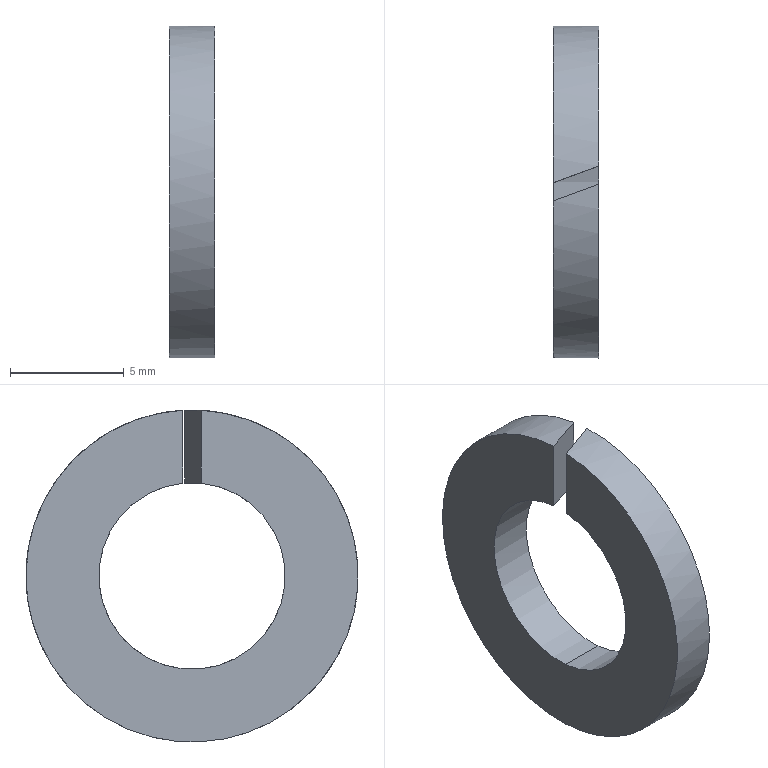Part | STEP file | KS B 1324 - No. 2 - 8 | 1 solid | 8 faces | box 2 x 14.6 x 14.6 mm | volume 224.071 mm3 | cylinder 4 | plane 4 | commonest cylinder face diameters 8.2 x2 14.6 x2
STEP:
#1=CARTESIAN_POINT('',(0.,0.,0.));
#2=DIRECTION('',(0.,0.,1.));
#3=DIRECTION('',(1.,0.,0.));
#4=AXIS2_PLACEMENT_3D('',#1,#2,#3);
#5=CARTESIAN_POINT('',(2.,1.128,3.942));
#6=VERTEX_POINT('',#5);
#7=CARTESIAN_POINT('',(0.,0.4,4.08));
#8=VERTEX_POINT('',#7);
#9=CARTESIAN_POINT('',(2.,1.128,3.942));
#10=CARTESIAN_POINT('',(1.346,0.8898,4.01));
#11=CARTESIAN_POINT('',(0.6773,0.6465,4.056));
#12=CARTESIAN_POINT('',(0.,0.4,4.08));
#13=(BOUNDED_CURVE()B_SPLINE_CURVE(3,(#9,#10,#11,#12),.UNSPECIFIED.,.F.,.F.)B_SPLINE_CURVE_WITH_KNOTS((4,4),(4.434,4.615),.PIECEWISE_BEZIER_KNOTS.)CURVE()GEOMETRIC_REPRESENTATION_ITEM()RATIONAL_B_SPLINE_CURVE((1.,0.9973,0.9973,1.))REPRESENTATION_ITEM(''));
#14=CARTESIAN_POINT('',(0.,0.,0.));
#15=DIRECTION('',(1.,0.,0.));
#16=DIRECTION('',(0.,-0.08878,-0.9961));
#17=AXIS2_PLACEMENT_3D('',#14,#15,#16);
#18=CYLINDRICAL_SURFACE('',#17,4.1);
#19=CARTESIAN_POINT('',(2.952,2.));
#20=CARTESIAN_POINT('',(2.955,1.97));
#21=CARTESIAN_POINT('',(2.96,1.911));
#22=CARTESIAN_POINT('',(2.968,1.822));
#23=CARTESIAN_POINT('',(2.976,1.732));
#24=CARTESIAN_POINT('',(2.985,1.642));
#25=CARTESIAN_POINT('',(2.993,1.552));
#26=CARTESIAN_POINT('',(3.001,1.462));
#27=CARTESIAN_POINT('',(3.009,1.372));
#28=CARTESIAN_POINT('',(3.018,1.281));
#29=CARTESIAN_POINT('',(3.026,1.191));
#30=CARTESIAN_POINT('',(3.034,1.1));
#31=CARTESIAN_POINT('',(3.042,1.009));
#32=CARTESIAN_POINT('',(3.051,0.9175));
#33=CARTESIAN_POINT('',(3.059,0.8262));
#34=CARTESIAN_POINT('',(3.067,0.7348));
#35=CARTESIAN_POINT('',(3.075,0.6432));
#36=CARTESIAN_POINT('',(3.083,0.5516));
#37=CARTESIAN_POINT('',(3.092,0.4598));
#38=CARTESIAN_POINT('',(3.1,0.368));
#39=CARTESIAN_POINT('',(3.108,0.2761));
#40=CARTESIAN_POINT('',(3.116,0.1841));
#41=CARTESIAN_POINT('',(3.125,0.09209));
#42=CARTESIAN_POINT('',(3.13,0.0307));
#43=CARTESIAN_POINT('',(3.133,0.));
#44=B_SPLINE_CURVE_WITH_KNOTS('',3,(#19,#20,#21,#22,#23,#24,#25,#26,#27,#28,#29,#30,#31,#32,#33,#34,#35,#36,#37,#38,#39,#40,#41,#42,#43),.UNSPECIFIED.,.F.,.F.,(4,1,1,1,1,1,1,1,1,1,1,1,1,1,1,1,1,1,1,1,1,1,4),(4.434,4.442,4.45,4.458,4.467,4.475,4.483,4.491,4.5,4.508,4.516,4.524,4.532,4.541,4.549,4.557,4.565,4.574,4.582,4.59,4.598,4.606,4.615),.QUASI_UNIFORM_KNOTS.);
#45=(GEOMETRIC_REPRESENTATION_CONTEXT(2)PARAMETRIC_REPRESENTATION_CONTEXT()REPRESENTATION_CONTEXT('',''));
#46=DEFINITIONAL_REPRESENTATION('',(#44),#45);
#47=PCURVE('',#18,#46);
#48=CARTESIAN_POINT('',(0.,0.4,0.));
#49=DIRECTION('',(-0.342,0.9397,0.));
#50=DIRECTION('',(0.,0.,1.));
#51=AXIS2_PLACEMENT_3D('',#48,#49,#50);
#52=PLANE('',#51);
#53=CARTESIAN_POINT('',(3.942,2.128));
#54=CARTESIAN_POINT('',(4.01,1.432));
#55=CARTESIAN_POINT('',(4.056,0.7207));
#56=CARTESIAN_POINT('',(4.08,0.));
#57=(BOUNDED_CURVE()B_SPLINE_CURVE(3,(#53,#54,#55,#56),.UNSPECIFIED.,.F.,.F.)B_SPLINE_CURVE_WITH_KNOTS((4,4),(4.434,4.615),.PIECEWISE_BEZIER_KNOTS.)CURVE()GEOMETRIC_REPRESENTATION_ITEM()RATIONAL_B_SPLINE_CURVE((1.,0.9973,0.9973,1.))REPRESENTATION_ITEM(''));
#58=(GEOMETRIC_REPRESENTATION_CONTEXT(2)PARAMETRIC_REPRESENTATION_CONTEXT()REPRESENTATION_CONTEXT('',''));
#59=DEFINITIONAL_REPRESENTATION('',(#57),#58);
#60=PCURVE('',#52,#59);
#61=SURFACE_CURVE('',#13,(#47,#60),.PCURVE_S1.);
#62=EDGE_CURVE('',#6,#8,#61,.T.);
#63=ORIENTED_EDGE('',*,*,#62,.F.);
#64=CARTESIAN_POINT('',(2.,-0.364,-4.084));
#65=VERTEX_POINT('',#64);
#66=CARTESIAN_POINT('',(2.,0.,0.));
#67=DIRECTION('',(-1.,0.,0.));
#68=DIRECTION('',(0.,-1.,0.));
#69=AXIS2_PLACEMENT_3D('',#66,#67,#68);
#70=CIRCLE('',#69,4.1);
#71=CARTESIAN_POINT('',(4.801,2.));
#72=DIRECTION('',(-1.,0.));
#73=VECTOR('',#72,1.);
#74=LINE('',#71,#73);
#75=(GEOMETRIC_REPRESENTATION_CONTEXT(2)PARAMETRIC_REPRESENTATION_CONTEXT()REPRESENTATION_CONTEXT('',''));
#76=DEFINITIONAL_REPRESENTATION('',(#74),#75);
#77=PCURVE('',#18,#76);
#78=CARTESIAN_POINT('',(2.,0.,0.));
#79=DIRECTION('',(-1.,0.,0.));
#80=DIRECTION('',(0.,0.,1.));
#81=AXIS2_PLACEMENT_3D('',#78,#79,#80);
#82=PLANE('',#81);
#83=CARTESIAN_POINT('',(0.,0.));
#84=DIRECTION('',(0.,-1.));
#85=AXIS2_PLACEMENT_2D('',#83,#84);
#86=CIRCLE('',#85,4.1);
#87=(GEOMETRIC_REPRESENTATION_CONTEXT(2)PARAMETRIC_REPRESENTATION_CONTEXT()REPRESENTATION_CONTEXT('',''));
#88=DEFINITIONAL_REPRESENTATION('',(#86),#87);
#89=PCURVE('',#82,#88);
#90=SURFACE_CURVE('',#70,(#77,#89),.PCURVE_S1.);
#91=EDGE_CURVE('',#6,#65,#90,.T.);
#92=ORIENTED_EDGE('',*,*,#91,.T.);
#93=CARTESIAN_POINT('',(0.,-0.364,-4.084));
#94=VERTEX_POINT('',#93);
#95=CARTESIAN_POINT('',(0.,-0.364,-4.084));
#96=DIRECTION('',(1.,0.,0.));
#97=VECTOR('',#96,1.);
#98=LINE('',#95,#97);
#99=CARTESIAN_POINT('',(0.,0.));
#100=DIRECTION('',(0.,1.));
#101=VECTOR('',#100,1.);
#102=LINE('',#99,#101);
#103=(GEOMETRIC_REPRESENTATION_CONTEXT(2)PARAMETRIC_REPRESENTATION_CONTEXT()REPRESENTATION_CONTEXT('',''));
#104=DEFINITIONAL_REPRESENTATION('',(#102),#103);
#105=PCURVE('',#18,#104);
#106=CARTESIAN_POINT('',(0.,0.,0.));
#107=DIRECTION('',(1.,0.,0.));
#108=DIRECTION('',(0.,-0.08878,-0.9961));
#109=AXIS2_PLACEMENT_3D('',#106,#107,#108);
#110=CYLINDRICAL_SURFACE('',#109,4.1);
#111=CARTESIAN_POINT('',(6.283,0.));
#112=DIRECTION('',(0.,1.));
#113=VECTOR('',#112,1.);
#114=LINE('',#111,#113);
#115=(GEOMETRIC_REPRESENTATION_CONTEXT(2)PARAMETRIC_REPRESENTATION_CONTEXT()REPRESENTATION_CONTEXT('',''));
#116=DEFINITIONAL_REPRESENTATION('',(#114),#115);
#117=PCURVE('',#110,#116);
#118=SURFACE_CURVE('',#98,(#105,#117),.PCURVE_S1.);
#119=EDGE_CURVE('',#94,#65,#118,.T.);
#120=ORIENTED_EDGE('',*,*,#119,.F.);
#121=CARTESIAN_POINT('',(0.,0.,0.));
#122=DIRECTION('',(1.,0.,0.));
#123=DIRECTION('',(0.,-1.,0.));
#124=AXIS2_PLACEMENT_3D('',#121,#122,#123);
#125=CIRCLE('',#124,4.1);
#126=CARTESIAN_POINT('',(-1.482,0.));
#127=DIRECTION('',(1.,0.));
#128=VECTOR('',#127,1.);
#129=LINE('',#126,#128);
#130=(GEOMETRIC_REPRESENTATION_CONTEXT(2)PARAMETRIC_REPRESENTATION_CONTEXT()REPRESENTATION_CONTEXT('',''));
#131=DEFINITIONAL_REPRESENTATION('',(#129),#130);
#132=PCURVE('',#18,#131);
#133=CARTESIAN_POINT('',(0.,0.,0.));
#134=DIRECTION('',(-1.,0.,0.));
#135=DIRECTION('',(0.,0.,1.));
#136=AXIS2_PLACEMENT_3D('',#133,#134,#135);
#137=PLANE('',#136);
#138=CARTESIAN_POINT('',(0.,-4.1));
#139=CARTESIAN_POINT('',(-7.101,-4.1));
#140=CARTESIAN_POINT('',(-3.551,2.05));
#141=CARTESIAN_POINT('',(0.,8.2));
#142=CARTESIAN_POINT('',(3.551,2.05));
#143=CARTESIAN_POINT('',(7.101,-4.1));
#144=CARTESIAN_POINT('',(0.,-4.1));
#145=(BOUNDED_CURVE()B_SPLINE_CURVE(2,(#138,#139,#140,#141,#142,#143,#144),.UNSPECIFIED.,.T.,.F.)B_SPLINE_CURVE_WITH_KNOTS((1,2,2,2,2,1),(-2.094,0.,2.094,4.189,6.283,8.378),.UNSPECIFIED.)CURVE()GEOMETRIC_REPRESENTATION_ITEM()RATIONAL_B_SPLINE_CURVE((1.,0.5,1.,0.5,1.,0.5,1.))REPRESENTATION_ITEM(''));
#146=(GEOMETRIC_REPRESENTATION_CONTEXT(2)PARAMETRIC_REPRESENTATION_CONTEXT()REPRESENTATION_CONTEXT('',''));
#147=DEFINITIONAL_REPRESENTATION('',(#145),#146);
#148=PCURVE('',#137,#147);
#149=SURFACE_CURVE('',#125,(#132,#148),.PCURVE_S1.);
#150=EDGE_CURVE('',#94,#8,#149,.T.);
#151=ORIENTED_EDGE('',*,*,#150,.T.);
#152=EDGE_LOOP('',(#63,#92,#120,#151));
#153=FACE_BOUND('',#152,.F.);
#154=ADVANCED_FACE('',(#153),#18,.F.);
#155=CARTESIAN_POINT('',(0.,-0.364,-7.291));
#156=VERTEX_POINT('',#155);
#157=CARTESIAN_POINT('',(0.,-0.4,7.289));
#158=VERTEX_POINT('',#157);
#159=CARTESIAN_POINT('',(0.,0.,0.));
#160=DIRECTION('',(-1.,0.,0.));
#161=DIRECTION('',(0.,-1.,0.));
#162=AXIS2_PLACEMENT_3D('',#159,#160,#161);
#163=CIRCLE('',#162,7.3);
#164=CARTESIAN_POINT('',(0.,0.,0.));
#165=DIRECTION('',(1.,0.,0.));
#166=DIRECTION('',(0.,-0.04986,-0.9988));
#167=AXIS2_PLACEMENT_3D('',#164,#165,#166);
#168=CYLINDRICAL_SURFACE('',#167,7.3);
#169=CARTESIAN_POINT('',(11.045,0.));
#170=DIRECTION('',(-1.,0.));
#171=VECTOR('',#170,1.);
#172=LINE('',#169,#171);
#173=(GEOMETRIC_REPRESENTATION_CONTEXT(2)PARAMETRIC_REPRESENTATION_CONTEXT()REPRESENTATION_CONTEXT('',''));
#174=DEFINITIONAL_REPRESENTATION('',(#172),#173);
#175=PCURVE('',#168,#174);
#176=CARTESIAN_POINT('',(0.,0.));
#177=DIRECTION('',(0.,-1.));
#178=AXIS2_PLACEMENT_2D('',#176,#177);
#179=CIRCLE('',#178,7.3);
#180=(GEOMETRIC_REPRESENTATION_CONTEXT(2)PARAMETRIC_REPRESENTATION_CONTEXT()REPRESENTATION_CONTEXT('',''));
#181=DEFINITIONAL_REPRESENTATION('',(#179),#180);
#182=PCURVE('',#137,#181);
#183=SURFACE_CURVE('',#163,(#175,#182),.PCURVE_S1.);
#184=EDGE_CURVE('',#156,#158,#183,.T.);
#185=ORIENTED_EDGE('',*,*,#184,.F.);
#186=CARTESIAN_POINT('',(2.,-0.364,-7.291));
#187=VERTEX_POINT('',#186);
#188=CARTESIAN_POINT('',(0.,-0.364,-7.291));
#189=DIRECTION('',(1.,0.,0.));
#190=VECTOR('',#189,1.);
#191=LINE('',#188,#190);
#192=CARTESIAN_POINT('',(6.283,0.));
#193=DIRECTION('',(0.,1.));
#194=VECTOR('',#193,1.);
#195=LINE('',#192,#194);
#196=(GEOMETRIC_REPRESENTATION_CONTEXT(2)PARAMETRIC_REPRESENTATION_CONTEXT()REPRESENTATION_CONTEXT('',''));
#197=DEFINITIONAL_REPRESENTATION('',(#195),#196);
#198=PCURVE('',#168,#197);
#199=CARTESIAN_POINT('',(0.,0.,0.));
#200=DIRECTION('',(1.,0.,0.));
#201=DIRECTION('',(0.,-0.04986,-0.9988));
#202=AXIS2_PLACEMENT_3D('',#199,#200,#201);
#203=CYLINDRICAL_SURFACE('',#202,7.3);
#204=CARTESIAN_POINT('',(0.,0.));
#205=DIRECTION('',(0.,1.));
#206=VECTOR('',#205,1.);
#207=LINE('',#204,#206);
#208=(GEOMETRIC_REPRESENTATION_CONTEXT(2)PARAMETRIC_REPRESENTATION_CONTEXT()REPRESENTATION_CONTEXT('',''));
#209=DEFINITIONAL_REPRESENTATION('',(#207),#208);
#210=PCURVE('',#203,#209);
#211=SURFACE_CURVE('',#191,(#198,#210),.PCURVE_S1.);
#212=EDGE_CURVE('',#156,#187,#211,.T.);
#213=ORIENTED_EDGE('',*,*,#212,.T.);
#214=CARTESIAN_POINT('',(2.,0.3279,7.293));
#215=VERTEX_POINT('',#214);
#216=CARTESIAN_POINT('',(2.,0.,0.));
#217=DIRECTION('',(-1.,0.,0.));
#218=DIRECTION('',(0.,-1.,0.));
#219=AXIS2_PLACEMENT_3D('',#216,#217,#218);
#220=CIRCLE('',#219,7.3);
#221=CARTESIAN_POINT('',(11.045,2.));
#222=DIRECTION('',(-1.,0.));
#223=VECTOR('',#222,1.);
#224=LINE('',#221,#223);
#225=(GEOMETRIC_REPRESENTATION_CONTEXT(2)PARAMETRIC_REPRESENTATION_CONTEXT()REPRESENTATION_CONTEXT('',''));
#226=DEFINITIONAL_REPRESENTATION('',(#224),#225);
#227=PCURVE('',#168,#226);
#228=CARTESIAN_POINT('',(0.,0.));
#229=DIRECTION('',(0.,-1.));
#230=AXIS2_PLACEMENT_2D('',#228,#229);
#231=CIRCLE('',#230,7.3);
#232=(GEOMETRIC_REPRESENTATION_CONTEXT(2)PARAMETRIC_REPRESENTATION_CONTEXT()REPRESENTATION_CONTEXT('',''));
#233=DEFINITIONAL_REPRESENTATION('',(#231),#232);
#234=PCURVE('',#82,#233);
#235=SURFACE_CURVE('',#220,(#227,#234),.PCURVE_S1.);
#236=EDGE_CURVE('',#187,#215,#235,.T.);
#237=ORIENTED_EDGE('',*,*,#236,.T.);
#238=CARTESIAN_POINT('',(2.,0.3279,7.293));
#239=CARTESIAN_POINT('',(1.333,0.08533,7.304));
#240=CARTESIAN_POINT('',(0.6662,-0.1575,7.302));
#241=CARTESIAN_POINT('',(0.,-0.4,7.289));
#242=(BOUNDED_CURVE()B_SPLINE_CURVE(3,(#238,#239,#240,#241),.UNSPECIFIED.,.F.,.F.)B_SPLINE_CURVE_WITH_KNOTS((4,4),(4.667,4.767),.PIECEWISE_BEZIER_KNOTS.)CURVE()GEOMETRIC_REPRESENTATION_ITEM()RATIONAL_B_SPLINE_CURVE((1.,0.9992,0.9992,1.))REPRESENTATION_ITEM(''));
#243=CARTESIAN_POINT('',(3.147,2.));
#244=CARTESIAN_POINT('',(3.148,1.97));
#245=CARTESIAN_POINT('',(3.151,1.909));
#246=CARTESIAN_POINT('',(3.156,1.818));
#247=CARTESIAN_POINT('',(3.16,1.727));
#248=CARTESIAN_POINT('',(3.165,1.637));
#249=CARTESIAN_POINT('',(3.169,1.546));
#250=CARTESIAN_POINT('',(3.174,1.455));
#251=CARTESIAN_POINT('',(3.178,1.364));
#252=CARTESIAN_POINT('',(3.183,1.273));
#253=CARTESIAN_POINT('',(3.187,1.182));
#254=CARTESIAN_POINT('',(3.192,1.091));
#255=CARTESIAN_POINT('',(3.196,0.9999));
#256=CARTESIAN_POINT('',(3.201,0.9089));
#257=CARTESIAN_POINT('',(3.205,0.818));
#258=CARTESIAN_POINT('',(3.21,0.727));
#259=CARTESIAN_POINT('',(3.215,0.6361));
#260=CARTESIAN_POINT('',(3.219,0.5451));
#261=CARTESIAN_POINT('',(3.224,0.4542));
#262=CARTESIAN_POINT('',(3.228,0.3633));
#263=CARTESIAN_POINT('',(3.233,0.2725));
#264=CARTESIAN_POINT('',(3.237,0.1816));
#265=CARTESIAN_POINT('',(3.242,0.09078));
#266=CARTESIAN_POINT('',(3.245,0.03026));
#267=CARTESIAN_POINT('',(3.246,0.));
#268=B_SPLINE_CURVE_WITH_KNOTS('',3,(#243,#244,#245,#246,#247,#248,#249,#250,#251,#252,#253,#254,#255,#256,#257,#258,#259,#260,#261,#262,#263,#264,#265,#266,#267),.UNSPECIFIED.,.F.,.F.,(4,1,1,1,1,1,1,1,1,1,1,1,1,1,1,1,1,1,1,1,1,1,4),(4.667,4.672,4.677,4.681,4.686,4.69,4.695,4.699,4.704,4.708,4.713,4.717,4.722,4.726,4.731,4.735,4.74,4.745,4.749,4.754,4.758,4.763,4.767),.QUASI_UNIFORM_KNOTS.);
#269=(GEOMETRIC_REPRESENTATION_CONTEXT(2)PARAMETRIC_REPRESENTATION_CONTEXT()REPRESENTATION_CONTEXT('',''));
#270=DEFINITIONAL_REPRESENTATION('',(#268),#269);
#271=PCURVE('',#168,#270);
#272=CARTESIAN_POINT('',(2.,0.3279,0.));
#273=DIRECTION('',(0.342,-0.9397,0.));
#274=DIRECTION('',(0.,0.,-1.));
#275=AXIS2_PLACEMENT_3D('',#272,#273,#274);
#276=PLANE('',#275);
#277=CARTESIAN_POINT('',(-7.293,0.));
#278=CARTESIAN_POINT('',(-7.304,-0.7093));
#279=CARTESIAN_POINT('',(-7.302,-1.419));
#280=CARTESIAN_POINT('',(-7.289,-2.128));
#281=(BOUNDED_CURVE()B_SPLINE_CURVE(3,(#277,#278,#279,#280),.UNSPECIFIED.,.F.,.F.)B_SPLINE_CURVE_WITH_KNOTS((4,4),(4.667,4.767),.PIECEWISE_BEZIER_KNOTS.)CURVE()GEOMETRIC_REPRESENTATION_ITEM()RATIONAL_B_SPLINE_CURVE((1.,0.9992,0.9992,1.))REPRESENTATION_ITEM(''));
#282=(GEOMETRIC_REPRESENTATION_CONTEXT(2)PARAMETRIC_REPRESENTATION_CONTEXT()REPRESENTATION_CONTEXT('',''));
#283=DEFINITIONAL_REPRESENTATION('',(#281),#282);
#284=PCURVE('',#276,#283);
#285=SURFACE_CURVE('',#242,(#271,#284),.PCURVE_S1.);
#286=EDGE_CURVE('',#215,#158,#285,.T.);
#287=ORIENTED_EDGE('',*,*,#286,.T.);
#288=EDGE_LOOP('',(#185,#213,#237,#287));
#289=FACE_BOUND('',#288,.T.);
#290=ADVANCED_FACE('',(#289),#168,.T.);
#291=CARTESIAN_POINT('',(0.,-0.4,4.08));
#292=VERTEX_POINT('',#291);
#293=CARTESIAN_POINT('',(0.,-0.4,0.));
#294=DIRECTION('',(0.,0.,-1.));
#295=VECTOR('',#294,1.);
#296=LINE('',#293,#295);
#297=CARTESIAN_POINT('',(0.,-0.4));
#298=DIRECTION('',(-1.,0.));
#299=VECTOR('',#298,1.);
#300=LINE('',#297,#299);
#301=(GEOMETRIC_REPRESENTATION_CONTEXT(2)PARAMETRIC_REPRESENTATION_CONTEXT()REPRESENTATION_CONTEXT('',''));
#302=DEFINITIONAL_REPRESENTATION('',(#300),#301);
#303=PCURVE('',#137,#302);
#304=CARTESIAN_POINT('',(0.,-2.128));
#305=DIRECTION('',(1.,0.));
#306=VECTOR('',#305,1.);
#307=LINE('',#304,#306);
#308=(GEOMETRIC_REPRESENTATION_CONTEXT(2)PARAMETRIC_REPRESENTATION_CONTEXT()REPRESENTATION_CONTEXT('',''));
#309=DEFINITIONAL_REPRESENTATION('',(#307),#308);
#310=PCURVE('',#276,#309);
#311=SURFACE_CURVE('',#296,(#303,#310),.PCURVE_S1.);
#312=EDGE_CURVE('',#158,#292,#311,.T.);
#313=ORIENTED_EDGE('',*,*,#312,.T.);
#314=CARTESIAN_POINT('',(0.,0.,0.));
#315=DIRECTION('',(1.,0.,0.));
#316=DIRECTION('',(0.,-1.,0.));
#317=AXIS2_PLACEMENT_3D('',#314,#315,#316);
#318=CIRCLE('',#317,4.1);
#319=CARTESIAN_POINT('',(0.,-4.1));
#320=CARTESIAN_POINT('',(-7.101,-4.1));
#321=CARTESIAN_POINT('',(-3.551,2.05));
#322=CARTESIAN_POINT('',(0.,8.2));
#323=CARTESIAN_POINT('',(3.551,2.05));
#324=CARTESIAN_POINT('',(7.101,-4.1));
#325=CARTESIAN_POINT('',(0.,-4.1));
#326=(BOUNDED_CURVE()B_SPLINE_CURVE(2,(#319,#320,#321,#322,#323,#324,#325),.UNSPECIFIED.,.T.,.F.)B_SPLINE_CURVE_WITH_KNOTS((1,2,2,2,2,1),(-2.094,0.,2.094,4.189,6.283,8.378),.UNSPECIFIED.)CURVE()GEOMETRIC_REPRESENTATION_ITEM()RATIONAL_B_SPLINE_CURVE((1.,0.5,1.,0.5,1.,0.5,1.))REPRESENTATION_ITEM(''));
#327=(GEOMETRIC_REPRESENTATION_CONTEXT(2)PARAMETRIC_REPRESENTATION_CONTEXT()REPRESENTATION_CONTEXT('',''));
#328=DEFINITIONAL_REPRESENTATION('',(#326),#327);
#329=PCURVE('',#137,#328);
#330=CARTESIAN_POINT('',(-1.482,0.));
#331=DIRECTION('',(1.,0.));
#332=VECTOR('',#331,1.);
#333=LINE('',#330,#332);
#334=(GEOMETRIC_REPRESENTATION_CONTEXT(2)PARAMETRIC_REPRESENTATION_CONTEXT()REPRESENTATION_CONTEXT('',''));
#335=DEFINITIONAL_REPRESENTATION('',(#333),#334);
#336=PCURVE('',#110,#335);
#337=SURFACE_CURVE('',#318,(#329,#336),.PCURVE_S1.);
#338=EDGE_CURVE('',#292,#94,#337,.T.);
#339=ORIENTED_EDGE('',*,*,#338,.T.);
#340=ORIENTED_EDGE('',*,*,#150,.T.);
#341=CARTESIAN_POINT('',(0.,0.4,7.289));
#342=VERTEX_POINT('',#341);
#343=CARTESIAN_POINT('',(0.,0.4,0.));
#344=DIRECTION('',(0.,0.,1.));
#345=VECTOR('',#344,1.);
#346=LINE('',#343,#345);
#347=CARTESIAN_POINT('',(0.,0.4));
#348=DIRECTION('',(1.,0.));
#349=VECTOR('',#348,1.);
#350=LINE('',#347,#349);
#351=(GEOMETRIC_REPRESENTATION_CONTEXT(2)PARAMETRIC_REPRESENTATION_CONTEXT()REPRESENTATION_CONTEXT('',''));
#352=DEFINITIONAL_REPRESENTATION('',(#350),#351);
#353=PCURVE('',#137,#352);
#354=CARTESIAN_POINT('',(0.,0.));
#355=DIRECTION('',(1.,0.));
#356=VECTOR('',#355,1.);
#357=LINE('',#354,#356);
#358=(GEOMETRIC_REPRESENTATION_CONTEXT(2)PARAMETRIC_REPRESENTATION_CONTEXT()REPRESENTATION_CONTEXT('',''));
#359=DEFINITIONAL_REPRESENTATION('',(#357),#358);
#360=PCURVE('',#52,#359);
#361=SURFACE_CURVE('',#346,(#353,#360),.PCURVE_S1.);
#362=EDGE_CURVE('',#8,#342,#361,.T.);
#363=ORIENTED_EDGE('',*,*,#362,.T.);
#364=CARTESIAN_POINT('',(0.,0.,0.));
#365=DIRECTION('',(-1.,0.,0.));
#366=DIRECTION('',(0.,-1.,0.));
#367=AXIS2_PLACEMENT_3D('',#364,#365,#366);
#368=CIRCLE('',#367,7.3);
#369=CARTESIAN_POINT('',(0.,0.));
#370=DIRECTION('',(0.,-1.));
#371=AXIS2_PLACEMENT_2D('',#369,#370);
#372=CIRCLE('',#371,7.3);
#373=(GEOMETRIC_REPRESENTATION_CONTEXT(2)PARAMETRIC_REPRESENTATION_CONTEXT()REPRESENTATION_CONTEXT('',''));
#374=DEFINITIONAL_REPRESENTATION('',(#372),#373);
#375=PCURVE('',#137,#374);
#376=CARTESIAN_POINT('',(4.762,0.));
#377=DIRECTION('',(-1.,0.));
#378=VECTOR('',#377,1.);
#379=LINE('',#376,#378);
#380=(GEOMETRIC_REPRESENTATION_CONTEXT(2)PARAMETRIC_REPRESENTATION_CONTEXT()REPRESENTATION_CONTEXT('',''));
#381=DEFINITIONAL_REPRESENTATION('',(#379),#380);
#382=PCURVE('',#203,#381);
#383=SURFACE_CURVE('',#368,(#375,#382),.PCURVE_S1.);
#384=EDGE_CURVE('',#342,#156,#383,.T.);
#385=ORIENTED_EDGE('',*,*,#384,.T.);
#386=ORIENTED_EDGE('',*,*,#184,.T.);
#387=EDGE_LOOP('',(#313,#339,#340,#363,#385,#386));
#388=FACE_BOUND('',#387,.T.);
#389=ADVANCED_FACE('',(#388),#137,.T.);
#390=ORIENTED_EDGE('',*,*,#212,.F.);
#391=ORIENTED_EDGE('',*,*,#384,.F.);
#392=CARTESIAN_POINT('',(2.,1.128,7.212));
#393=VERTEX_POINT('',#392);
#394=CARTESIAN_POINT('',(0.,0.4,7.289));
#395=CARTESIAN_POINT('',(0.6699,0.6438,7.276));
#396=CARTESIAN_POINT('',(1.337,0.8867,7.25));
#397=CARTESIAN_POINT('',(2.,1.128,7.212));
#398=(BOUNDED_CURVE()B_SPLINE_CURVE(3,(#394,#395,#396,#397),.UNSPECIFIED.,.F.,.F.)B_SPLINE_CURVE_WITH_KNOTS((4,4),(1.626,1.726),.PIECEWISE_BEZIER_KNOTS.)CURVE()GEOMETRIC_REPRESENTATION_ITEM()RATIONAL_B_SPLINE_CURVE((1.,0.9992,0.9992,1.))REPRESENTATION_ITEM(''));
#399=CARTESIAN_POINT('',(3.137,0.));
#400=CARTESIAN_POINT('',(3.135,0.03042));
#401=CARTESIAN_POINT('',(3.132,0.09127));
#402=CARTESIAN_POINT('',(3.128,0.1825));
#403=CARTESIAN_POINT('',(3.123,0.2738));
#404=CARTESIAN_POINT('',(3.118,0.365));
#405=CARTESIAN_POINT('',(3.114,0.4562));
#406=CARTESIAN_POINT('',(3.109,0.5473));
#407=CARTESIAN_POINT('',(3.105,0.6385));
#408=CARTESIAN_POINT('',(3.1,0.7296));
#409=CARTESIAN_POINT('',(3.096,0.8206));
#410=CARTESIAN_POINT('',(3.091,0.9117));
#411=CARTESIAN_POINT('',(3.086,1.003));
#412=CARTESIAN_POINT('',(3.082,1.094));
#413=CARTESIAN_POINT('',(3.077,1.184));
#414=CARTESIAN_POINT('',(3.073,1.275));
#415=CARTESIAN_POINT('',(3.068,1.366));
#416=CARTESIAN_POINT('',(3.064,1.457));
#417=CARTESIAN_POINT('',(3.059,1.548));
#418=CARTESIAN_POINT('',(3.055,1.638));
#419=CARTESIAN_POINT('',(3.05,1.729));
#420=CARTESIAN_POINT('',(3.045,1.819));
#421=CARTESIAN_POINT('',(3.041,1.91));
#422=CARTESIAN_POINT('',(3.038,1.97));
#423=CARTESIAN_POINT('',(3.036,2.));
#424=B_SPLINE_CURVE_WITH_KNOTS('',3,(#399,#400,#401,#402,#403,#404,#405,#406,#407,#408,#409,#410,#411,#412,#413,#414,#415,#416,#417,#418,#419,#420,#421,#422,#423),.UNSPECIFIED.,.F.,.F.,(4,1,1,1,1,1,1,1,1,1,1,1,1,1,1,1,1,1,1,1,1,1,4),(1.626,1.63,1.635,1.639,1.644,1.648,1.653,1.658,1.662,1.667,1.671,1.676,1.68,1.685,1.689,1.694,1.699,1.703,1.708,1.712,1.717,1.721,1.726),.QUASI_UNIFORM_KNOTS.);
#425=(GEOMETRIC_REPRESENTATION_CONTEXT(2)PARAMETRIC_REPRESENTATION_CONTEXT()REPRESENTATION_CONTEXT('',''));
#426=DEFINITIONAL_REPRESENTATION('',(#424),#425);
#427=PCURVE('',#203,#426);
#428=CARTESIAN_POINT('',(7.289,0.));
#429=CARTESIAN_POINT('',(7.276,0.7129));
#430=CARTESIAN_POINT('',(7.25,1.423));
#431=CARTESIAN_POINT('',(7.212,2.128));
#432=(BOUNDED_CURVE()B_SPLINE_CURVE(3,(#428,#429,#430,#431),.UNSPECIFIED.,.F.,.F.)B_SPLINE_CURVE_WITH_KNOTS((4,4),(1.626,1.726),.PIECEWISE_BEZIER_KNOTS.)CURVE()GEOMETRIC_REPRESENTATION_ITEM()RATIONAL_B_SPLINE_CURVE((1.,0.9992,0.9992,1.))REPRESENTATION_ITEM(''));
#433=(GEOMETRIC_REPRESENTATION_CONTEXT(2)PARAMETRIC_REPRESENTATION_CONTEXT()REPRESENTATION_CONTEXT('',''));
#434=DEFINITIONAL_REPRESENTATION('',(#432),#433);
#435=PCURVE('',#52,#434);
#436=SURFACE_CURVE('',#398,(#427,#435),.PCURVE_S1.);
#437=EDGE_CURVE('',#342,#393,#436,.T.);
#438=ORIENTED_EDGE('',*,*,#437,.T.);
#439=CARTESIAN_POINT('',(2.,0.,0.));
#440=DIRECTION('',(-1.,0.,0.));
#441=DIRECTION('',(0.,-1.,0.));
#442=AXIS2_PLACEMENT_3D('',#439,#440,#441);
#443=CIRCLE('',#442,7.3);
#444=CARTESIAN_POINT('',(4.762,2.));
#445=DIRECTION('',(-1.,0.));
#446=VECTOR('',#445,1.);
#447=LINE('',#444,#446);
#448=(GEOMETRIC_REPRESENTATION_CONTEXT(2)PARAMETRIC_REPRESENTATION_CONTEXT()REPRESENTATION_CONTEXT('',''));
#449=DEFINITIONAL_REPRESENTATION('',(#447),#448);
#450=PCURVE('',#203,#449);
#451=CARTESIAN_POINT('',(0.,0.));
#452=DIRECTION('',(0.,-1.));
#453=AXIS2_PLACEMENT_2D('',#451,#452);
#454=CIRCLE('',#453,7.3);
#455=(GEOMETRIC_REPRESENTATION_CONTEXT(2)PARAMETRIC_REPRESENTATION_CONTEXT()REPRESENTATION_CONTEXT('',''));
#456=DEFINITIONAL_REPRESENTATION('',(#454),#455);
#457=PCURVE('',#82,#456);
#458=SURFACE_CURVE('',#443,(#450,#457),.PCURVE_S1.);
#459=EDGE_CURVE('',#393,#187,#458,.T.);
#460=ORIENTED_EDGE('',*,*,#459,.T.);
#461=EDGE_LOOP('',(#390,#391,#438,#460));
#462=FACE_BOUND('',#461,.T.);
#463=ADVANCED_FACE('',(#462),#203,.T.);
#464=CARTESIAN_POINT('',(2.,0.3279,4.087));
#465=VERTEX_POINT('',#464);
#466=CARTESIAN_POINT('',(2.,0.,0.));
#467=DIRECTION('',(-1.,0.,0.));
#468=DIRECTION('',(0.,-1.,0.));
#469=AXIS2_PLACEMENT_3D('',#466,#467,#468);
#470=CIRCLE('',#469,4.1);
#471=CARTESIAN_POINT('',(11.084,2.));
#472=DIRECTION('',(-1.,0.));
#473=VECTOR('',#472,1.);
#474=LINE('',#471,#473);
#475=(GEOMETRIC_REPRESENTATION_CONTEXT(2)PARAMETRIC_REPRESENTATION_CONTEXT()REPRESENTATION_CONTEXT('',''));
#476=DEFINITIONAL_REPRESENTATION('',(#474),#475);
#477=PCURVE('',#110,#476);
#478=CARTESIAN_POINT('',(0.,0.));
#479=DIRECTION('',(0.,-1.));
#480=AXIS2_PLACEMENT_2D('',#478,#479);
#481=CIRCLE('',#480,4.1);
#482=(GEOMETRIC_REPRESENTATION_CONTEXT(2)PARAMETRIC_REPRESENTATION_CONTEXT()REPRESENTATION_CONTEXT('',''));
#483=DEFINITIONAL_REPRESENTATION('',(#481),#482);
#484=PCURVE('',#82,#483);
#485=SURFACE_CURVE('',#470,(#477,#484),.PCURVE_S1.);
#486=EDGE_CURVE('',#65,#465,#485,.T.);
#487=ORIENTED_EDGE('',*,*,#486,.T.);
#488=CARTESIAN_POINT('',(0.,-0.4,4.08));
#489=CARTESIAN_POINT('',(0.6653,-0.1579,4.104));
#490=CARTESIAN_POINT('',(1.334,0.08542,4.106));
#491=CARTESIAN_POINT('',(2.,0.3279,4.087));
#492=(BOUNDED_CURVE()B_SPLINE_CURVE(3,(#488,#489,#490,#491),.UNSPECIFIED.,.F.,.F.)B_SPLINE_CURVE_WITH_KNOTS((4,4),(1.473,1.651),.PIECEWISE_BEZIER_KNOTS.)CURVE()GEOMETRIC_REPRESENTATION_ITEM()RATIONAL_B_SPLINE_CURVE((1.,0.9974,0.9974,1.))REPRESENTATION_ITEM(''));
#493=CARTESIAN_POINT('',(3.328,0.));
#494=CARTESIAN_POINT('',(3.326,0.03016));
#495=CARTESIAN_POINT('',(3.32,0.09051));
#496=CARTESIAN_POINT('',(3.312,0.1811));
#497=CARTESIAN_POINT('',(3.304,0.2719));
#498=CARTESIAN_POINT('',(3.296,0.3626));
#499=CARTESIAN_POINT('',(3.288,0.4535));
#500=CARTESIAN_POINT('',(3.28,0.5444));
#501=CARTESIAN_POINT('',(3.272,0.6354));
#502=CARTESIAN_POINT('',(3.264,0.7264));
#503=CARTESIAN_POINT('',(3.255,0.8175));
#504=CARTESIAN_POINT('',(3.247,0.9085));
#505=CARTESIAN_POINT('',(3.239,0.9996));
#506=CARTESIAN_POINT('',(3.231,1.091));
#507=CARTESIAN_POINT('',(3.223,1.182));
#508=CARTESIAN_POINT('',(3.215,1.273));
#509=CARTESIAN_POINT('',(3.207,1.364));
#510=CARTESIAN_POINT('',(3.199,1.455));
#511=CARTESIAN_POINT('',(3.191,1.546));
#512=CARTESIAN_POINT('',(3.183,1.637));
#513=CARTESIAN_POINT('',(3.175,1.728));
#514=CARTESIAN_POINT('',(3.167,1.819));
#515=CARTESIAN_POINT('',(3.158,1.909));
#516=CARTESIAN_POINT('',(3.153,1.97));
#517=CARTESIAN_POINT('',(3.15,2.));
#518=B_SPLINE_CURVE_WITH_KNOTS('',3,(#493,#494,#495,#496,#497,#498,#499,#500,#501,#502,#503,#504,#505,#506,#507,#508,#509,#510,#511,#512,#513,#514,#515,#516,#517),.UNSPECIFIED.,.F.,.F.,(4,1,1,1,1,1,1,1,1,1,1,1,1,1,1,1,1,1,1,1,1,1,4),(1.473,1.481,1.489,1.497,1.505,1.513,1.522,1.53,1.538,1.546,1.554,1.562,1.57,1.578,1.586,1.594,1.602,1.61,1.619,1.627,1.635,1.643,1.651),.QUASI_UNIFORM_KNOTS.);
#519=(GEOMETRIC_REPRESENTATION_CONTEXT(2)PARAMETRIC_REPRESENTATION_CONTEXT()REPRESENTATION_CONTEXT('',''));
#520=DEFINITIONAL_REPRESENTATION('',(#518),#519);
#521=PCURVE('',#110,#520);
#522=CARTESIAN_POINT('',(-4.08,-2.128));
#523=CARTESIAN_POINT('',(-4.104,-1.42));
#524=CARTESIAN_POINT('',(-4.106,-0.7091));
#525=CARTESIAN_POINT('',(-4.087,0.));
#526=(BOUNDED_CURVE()B_SPLINE_CURVE(3,(#522,#523,#524,#525),.UNSPECIFIED.,.F.,.F.)B_SPLINE_CURVE_WITH_KNOTS((4,4),(1.473,1.651),.PIECEWISE_BEZIER_KNOTS.)CURVE()GEOMETRIC_REPRESENTATION_ITEM()RATIONAL_B_SPLINE_CURVE((1.,0.9974,0.9974,1.))REPRESENTATION_ITEM(''));
#527=(GEOMETRIC_REPRESENTATION_CONTEXT(2)PARAMETRIC_REPRESENTATION_CONTEXT()REPRESENTATION_CONTEXT('',''));
#528=DEFINITIONAL_REPRESENTATION('',(#526),#527);
#529=PCURVE('',#276,#528);
#530=SURFACE_CURVE('',#492,(#521,#529),.PCURVE_S1.);
#531=EDGE_CURVE('',#292,#465,#530,.T.);
#532=ORIENTED_EDGE('',*,*,#531,.F.);
#533=ORIENTED_EDGE('',*,*,#338,.T.);
#534=ORIENTED_EDGE('',*,*,#119,.T.);
#535=EDGE_LOOP('',(#487,#532,#533,#534));
#536=FACE_BOUND('',#535,.F.);
#537=ADVANCED_FACE('',(#536),#110,.F.);
#538=CARTESIAN_POINT('',(2.,0.3279,0.));
#539=DIRECTION('',(0.,0.,1.));
#540=VECTOR('',#539,1.);
#541=LINE('',#538,#540);
#542=CARTESIAN_POINT('',(0.,0.3279));
#543=DIRECTION('',(1.,0.));
#544=VECTOR('',#543,1.);
#545=LINE('',#542,#544);
#546=(GEOMETRIC_REPRESENTATION_CONTEXT(2)PARAMETRIC_REPRESENTATION_CONTEXT()REPRESENTATION_CONTEXT('',''));
#547=DEFINITIONAL_REPRESENTATION('',(#545),#546);
#548=PCURVE('',#82,#547);
#549=CARTESIAN_POINT('',(0.,0.));
#550=DIRECTION('',(-1.,0.));
#551=VECTOR('',#550,1.);
#552=LINE('',#549,#551);
#553=(GEOMETRIC_REPRESENTATION_CONTEXT(2)PARAMETRIC_REPRESENTATION_CONTEXT()REPRESENTATION_CONTEXT('',''));
#554=DEFINITIONAL_REPRESENTATION('',(#552),#553);
#555=PCURVE('',#276,#554);
#556=SURFACE_CURVE('',#541,(#548,#555),.PCURVE_S1.);
#557=EDGE_CURVE('',#465,#215,#556,.T.);
#558=ORIENTED_EDGE('',*,*,#557,.T.);
#559=ORIENTED_EDGE('',*,*,#236,.F.);
#560=ORIENTED_EDGE('',*,*,#459,.F.);
#561=CARTESIAN_POINT('',(2.,1.128,0.));
#562=DIRECTION('',(0.,0.,-1.));
#563=VECTOR('',#562,1.);
#564=LINE('',#561,#563);
#565=CARTESIAN_POINT('',(0.,1.128));
#566=DIRECTION('',(-1.,0.));
#567=VECTOR('',#566,1.);
#568=LINE('',#565,#567);
#569=(GEOMETRIC_REPRESENTATION_CONTEXT(2)PARAMETRIC_REPRESENTATION_CONTEXT()REPRESENTATION_CONTEXT('',''));
#570=DEFINITIONAL_REPRESENTATION('',(#568),#569);
#571=PCURVE('',#82,#570);
#572=CARTESIAN_POINT('',(0.,2.128));
#573=DIRECTION('',(-1.,0.));
#574=VECTOR('',#573,1.);
#575=LINE('',#572,#574);
#576=(GEOMETRIC_REPRESENTATION_CONTEXT(2)PARAMETRIC_REPRESENTATION_CONTEXT()REPRESENTATION_CONTEXT('',''));
#577=DEFINITIONAL_REPRESENTATION('',(#575),#576);
#578=PCURVE('',#52,#577);
#579=SURFACE_CURVE('',#564,(#571,#578),.PCURVE_S1.);
#580=EDGE_CURVE('',#393,#6,#579,.T.);
#581=ORIENTED_EDGE('',*,*,#580,.T.);
#582=ORIENTED_EDGE('',*,*,#91,.T.);
#583=ORIENTED_EDGE('',*,*,#486,.T.);
#584=EDGE_LOOP('',(#558,#559,#560,#581,#582,#583));
#585=FACE_BOUND('',#584,.T.);
#586=ADVANCED_FACE('',(#585),#82,.F.);
#587=ORIENTED_EDGE('',*,*,#531,.F.);
#588=ORIENTED_EDGE('',*,*,#312,.F.);
#589=ORIENTED_EDGE('',*,*,#286,.F.);
#590=ORIENTED_EDGE('',*,*,#557,.F.);
#591=EDGE_LOOP('',(#587,#588,#589,#590));
#592=FACE_BOUND('',#591,.T.);
#593=ADVANCED_FACE('',(#592),#276,.F.);
#594=ORIENTED_EDGE('',*,*,#62,.F.);
#595=ORIENTED_EDGE('',*,*,#580,.F.);
#596=ORIENTED_EDGE('',*,*,#437,.F.);
#597=ORIENTED_EDGE('',*,*,#362,.F.);
#598=EDGE_LOOP('',(#594,#595,#596,#597));
#599=FACE_BOUND('',#598,.T.);
#600=ADVANCED_FACE('',(#599),#52,.F.);
#601=CLOSED_SHELL('',(#154,#290,#389,#463,#537,#586,#593,#600));
#602=MANIFOLD_SOLID_BREP('',#601);
#603=(LENGTH_UNIT()NAMED_UNIT(*)SI_UNIT(.MILLI.,.METRE.));
#604=UNCERTAINTY_MEASURE_WITH_UNIT(LENGTH_MEASURE(0.0000001),#603,'','');
#605=(NAMED_UNIT(*)PLANE_ANGLE_UNIT()SI_UNIT($,.RADIAN.));
#606=(NAMED_UNIT(*)SI_UNIT($,.STERADIAN.)SOLID_ANGLE_UNIT());
#607=(GEOMETRIC_REPRESENTATION_CONTEXT(3)GLOBAL_UNCERTAINTY_ASSIGNED_CONTEXT((#604))GLOBAL_UNIT_ASSIGNED_CONTEXT((#603,#605,#606))REPRESENTATION_CONTEXT('',''));
#608=ADVANCED_BREP_SHAPE_REPRESENTATION('',(#4,#602),#607);